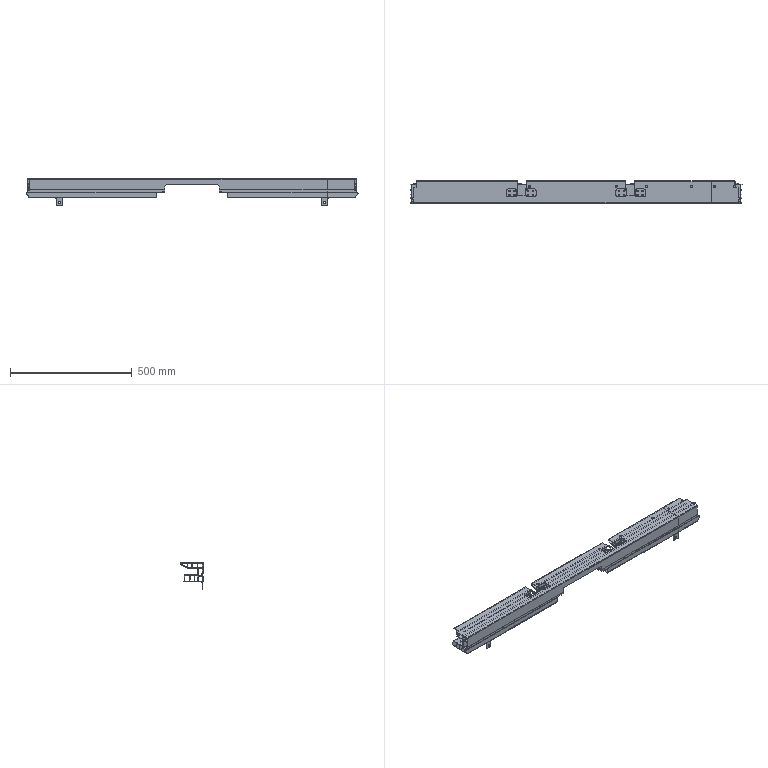NC program | NX | posted with a generic post | part box 1365 x 90.95 x 108.501 mm
Lines 17611 to 18323 of 23380:
(FIXED_CONTOUR , TOOL : R3)
N35190 T09 M6
N35192 G54
N35194 G17 G0 G90 X-536.016 Y-22.112 B0. C0. S9500 M3
N35196 G43 Z30. H9
N35198 Z-6.865
N35200 G94 G1 Z-11.665 F1000.
N35202 X-535.981 Y-22.077 Z-11.732 F2500.
N35204 X-535.904 Y-22. Z-11.861
N35206 X-535.813 Z-12.005
N35208 X-535.883 Y-22.071 Z-11.892
N35210 X-535.962 Y-22.15 Z-11.76
N35212 X-536.034 Y-22.222 Z-11.622
N35214 X-536.044 Y-22.287 Z-11.598
N35216 X-536.049 Y-22.329 Z-11.588
N35218 X-535.992 Y-22.271 Z-11.695
N35220 X-535.943 Y-22.223 Z-11.788
N35222 X-535.816 Y-22.096 Z-12.
N35224 X-535.721 Y-22. Z-12.146
N35226 X-535.696 Z-12.184
N35228 X-535.622 Z-12.282
N35230 X-535.696 Y-22.074 Z-12.182
N35232 X-535.756 Y-22.135 Z-12.087
N35234 X-535.816 Y-22.194 Z-12.
N35236 X-535.931 Y-22.31 Z-11.806
N35238 X-536.061 Y-22.44 Z-11.566
N35240 X-536.062 Y-22.536 Z-11.565
N35242 X-535.932 Y-22.406 Z-11.804
N35244 X-535.816 Y-22.29 Z-12.
N35246 X-535.727 Y-22.201 Z-12.131
N35248 X-535.696 Y-22.17 Z-12.179
N35250 X-535.576 Y-22.05 Z-12.341
N35252 X-535.526 Y-22. Z-12.398
N35254 X-535.427 Z-12.51
N35256 X-535.576 Y-22.149 Z-12.339
N35258 X-535.696 Y-22.269 Z-12.176
N35260 X-535.816 Y-22.389 Z-12.
N35262 X-535.934 Y-22.507 Z-11.802
N35264 X-536.062 Y-22.635 Z-11.564
N35266 Y-22.738
N35268 X-535.935 Y-22.611 Z-11.799
N35270 X-535.816 Y-22.493 Z-12.
N35272 X-535.696 Y-22.373 Z-12.176
N35274 X-535.576 Y-22.252 Z-12.336
N35276 X-535.33 Y-22.006 Z-12.618
N35278 X-535.323 Y-22. Z-12.625
N35280 X-535.213 Z-12.734
N35282 X-535.336 Y-22.122 Z-12.613
N35284 X-535.576 Y-22.362 Z-12.336
N35286 X-535.696 Y-22.483 Z-12.176
N35288 X-535.816 Y-22.603 Z-12.
N35290 X-535.936 Y-22.723 Z-11.797
N35292 X-536.062 Y-22.848 Z-11.564
N35294 Y-22.959 Z-11.563
N35296 X-535.936 Y-22.833 Z-11.796
N35298 X-535.816 Y-22.713 Z-12.
N35300 X-535.696 Y-22.593 Z-12.176
N35302 X-535.576 Y-22.473 Z-12.336
N35304 X-535.336 Y-22.232 Z-12.613
N35306 X-535.226 Y-22.123 Z-12.718
N35308 X-535.103 Y-22. Z-12.843
N35310 X-535.095 Z-12.851
N35312 X-534.993 Z-12.93
N35314 X-535.095 Y-22.102 Z-12.849
N35316 X-535.175 Y-22.182 Z-12.769
N35318 X-535.336 Y-22.343 Z-12.613
N35320 X-535.576 Y-22.583 Z-12.336
N35322 X-535.696 Y-22.703 Z-12.176
N35324 X-535.816 Y-22.823 Z-12.
N35326 X-535.936 Y-22.943 Z-11.796
N35328 X-536.062 Y-23.069 Z-11.563
N35330 Y-23.179 Z-11.564
N35332 X-535.936 Y-23.053 Z-11.796
N35334 X-535.816 Y-22.933 Z-12.
N35336 X-535.696 Y-22.813 Z-12.176
N35338 X-535.576 Y-22.693 Z-12.336
N35340 X-535.336 Y-22.453 Z-12.613
N35342 X-535.095 Y-22.212 Z-12.847
N35344 X-534.883 Y-22. Z-13.016
N35346 X-534.773 Z-13.096
N35348 X-534.855 Y-22.082 Z-13.037
N35350 X-535.095 Y-22.322 Z-12.845
N35352 X-535.336 Y-22.563 Z-12.613
N35354 X-535.576 Y-22.803 Z-12.336
N35356 X-535.696 Y-22.923 Z-12.176
N35358 X-535.816 Y-23.043 Z-12.
N35360 X-535.936 Y-23.163 Z-11.796
N35362 X-536.061 Y-23.289 Z-11.564
N35364 Y-23.398 Z-11.565
N35366 X-535.936 Y-23.273 Z-11.797
N35368 X-535.816 Y-23.153 Z-12.
N35370 X-535.696 Y-23.033 Z-12.176
N35372 X-535.576 Y-22.913 Z-12.336
N35374 X-535.336 Y-22.672 Z-12.613
N35376 X-535.095 Y-22.432 Z-12.845
N35378 X-534.855 Y-22.192 Z-13.037
N35380 X-534.765 Y-22.102 Z-13.1
N35382 X-534.663 Y-21.999 Z-13.175
N35384 X-534.615 Z-13.209
N35386 X-534.553 Z-13.246
N35388 X-534.615 Y-22.061 Z-13.208
N35390 X-534.714 Y-22.16 Z-13.135
N35392 X-534.855 Y-22.301 Z-13.037
N35394 X-535.095 Y-22.541 Z-12.845
N35396 X-535.336 Y-22.782 Z-12.613
N35398 X-535.576 Y-23.022 Z-12.336
N35400 X-535.696 Y-23.142 Z-12.176
N35402 X-535.816 Y-23.262 Z-12.
N35404 X-535.935 Y-23.381 Z-11.799
N35406 X-536.061 Y-23.507 Z-11.566
N35408 Y-23.572
N35410 X-536.058 Y-23.614 Z-11.573
N35412 X-535.934 Y-23.489 Z-11.801
N35414 X-535.816 Y-23.372 Z-12.
N35416 X-535.696 Y-23.252 Z-12.176
N35418 X-535.576 Y-23.132 Z-12.336
N35420 X-535.336 Y-22.891 Z-12.613
N35422 X-535.095 Y-22.651 Z-12.845
N35424 X-534.855 Y-22.411 Z-13.037
N35426 X-534.662 Y-22.218 Z-13.171
N35428 X-534.615 Y-22.17 Z-13.206
N35430 X-534.441 Y-21.997 Z-13.311
N35432 X-534.33 Y-21.996 Z-13.375
N35434 X-534.374 Y-22.04 Z-13.351
N35436 X-534.615 Y-22.28 Z-13.204
N35438 X-534.855 Y-22.521 Z-13.037
N35440 X-535.095 Y-22.761 Z-12.845
N35442 X-535.336 Y-23.001 Z-12.613
N35444 X-535.576 Y-23.241 Z-12.336
N35446 X-535.696 Y-23.362 Z-12.176
N35448 X-535.816 Y-23.482 Z-12.
N35450 X-535.933 Y-23.598 Z-11.803
N35452 X-536.046 Y-23.712 Z-11.594
N35454 X-536.031 Y-23.804 Z-11.63
N35456 X-535.931 Y-23.705 Z-11.805
N35458 X-535.816 Y-23.589 Z-12.
N35460 X-535.696 Y-23.469 Z-12.176
N35462 X-535.576 Y-23.349 Z-12.336
N35464 X-535.336 Y-23.109 Z-12.613
N35466 X-535.095 Y-22.868 Z-12.845
N35468 X-534.855 Y-22.628 Z-13.037
N35470 X-534.615 Y-22.388 Z-13.204
N35472 X-534.374 Y-22.147 Z-13.351
N35474 X-534.304 Y-22.077 Z-13.386
N35476 X-534.221 Y-21.994 Z-13.432
N35478 X-534.134 Y-21.993 Z-13.475
N35480 X-534.11 Y-21.991 Z-13.486
N35482 X-534.219 Y-22.1 Z-13.431
N35484 X-534.254 Y-22.134 Z-13.411
N35486 X-534.374 Y-22.255 Z-13.351
N35488 X-534.615 Y-22.495 Z-13.204
N35490 X-534.855 Y-22.735 Z-13.037
N35492 X-535.095 Y-22.976 Z-12.845
N35494 X-535.336 Y-23.216 Z-12.613
N35496 X-535.576 Y-23.456 Z-12.336
N35498 X-535.696 Y-23.576 Z-12.176
N35500 X-535.816 Y-23.697 Z-12.
N35502 X-535.914 Y-23.795 Z-11.836
N35504 X-535.962 Y-23.842 Z-11.76
N35506 X-536.007 Y-23.887 Z-11.682
N35508 X-536.003 Y-23.899 Z-11.689
N35510 X-535.97 Y-23.96 Z-11.752
N35512 X-535.893 Y-23.883 Z-11.874
N35514 X-535.873 Y-23.863 Z-11.903
N35516 X-535.816 Y-23.806 Z-12.
N35518 X-535.696 Y-23.686 Z-12.176
N35520 X-535.576 Y-23.565 Z-12.336
N35522 X-535.336 Y-23.325 Z-12.613
N35524 X-535.095 Y-23.085 Z-12.845
N35526 X-534.855 Y-22.845 Z-13.037
N35528 X-534.615 Y-22.604 Z-13.204
N35530 X-534.374 Y-22.364 Z-13.351
N35532 X-534.203 Y-22.193 Z-13.436
N35534 X-534.134 Y-22.124 Z-13.473
N35536 X-533.993 Y-21.982 Z-13.54
N35538 X-533.873 Y-21.974 Z-13.589
N35540 X-533.894 Y-21.995 Z-13.581
N35542 X-534.146 Y-22.247 Z-13.465
N35544 X-534.374 Y-22.475 Z-13.351
N35546 X-534.615 Y-22.716 Z-13.204
N35548 X-534.855 Y-22.956 Z-13.037
N35550 X-535.095 Y-23.196 Z-12.845
N35552 X-535.336 Y-23.436 Z-12.613
N35554 X-535.576 Y-23.677 Z-12.336
N35556 X-535.696 Y-23.797 Z-12.178
N35558 X-535.816 Y-23.917 Z-12.
N35560 X-535.841 Y-23.941 Z-11.959
N35562 X-535.899 Y-24. Z-11.869
N35564 X-535.786 Z-12.045
N35566 X-535.696 Y-23.91 Z-12.181
N35568 X-535.576 Y-23.79 Z-12.337
N35570 X-535.336 Y-23.549 Z-12.613
N35572 X-535.095 Y-23.309 Z-12.845
N35574 X-534.855 Y-23.069 Z-13.037
N35576 X-534.615 Y-22.828 Z-13.204
N35578 X-534.374 Y-22.588 Z-13.351
N35580 X-534.109 Y-22.322 Z-13.482
N35582 X-533.894 Y-22.108 Z-13.58
N35584 X-533.751 Y-21.965 Z-13.633
N35586 X-533.653 Y-21.957 Z-13.669
N35588 X-533.617 Y-21.946 Z-13.678
N35590 X-533.653 Y-21.982 Z-13.668
N35592 X-533.894 Y-22.223 Z-13.58
N35594 X-534.134 Y-22.463 Z-13.47
N35596 X-534.374 Y-22.703 Z-13.351
N35598 X-534.615 Y-22.944 Z-13.204
N35600 X-534.855 Y-23.184 Z-13.037
N35602 X-535.095 Y-23.424 Z-12.845
N35604 X-535.336 Y-23.665 Z-12.613
N35606 X-535.492 Y-23.821 Z-12.433
N35608 X-535.576 Y-23.905 Z-12.34
N35610 X-535.671 Y-24. Z-12.217
N35612 X-535.576 Z-12.342
N35614 X-535.563 Z-12.356
N35616 X-535.441 Y-23.878 Z-12.491
N35618 X-535.336 Y-23.772 Z-12.613
N35620 X-535.095 Y-23.532 Z-12.845
N35622 X-534.855 Y-23.292 Z-13.037
N35624 X-534.615 Y-23.051 Z-13.204
N35626 X-534.374 Y-22.811 Z-13.351
N35628 X-534.134 Y-22.571 Z-13.47
N35630 X-533.894 Y-22.33 Z-13.579
N35632 X-533.653 Y-22.09 Z-13.667
N35634 X-533.46 Y-21.897 Z-13.72
N35636 X-533.413 Y-21.882 Z-13.732
N35638 X-533.304 Y-21.849 Z-13.755
N35640 X-533.413 Y-21.958 Z-13.732
N35642 X-533.653 Y-22.198 Z-13.666
N35644 X-533.894 Y-22.439 Z-13.579
N35646 X-534.134 Y-22.679 Z-13.47
N35648 X-534.374 Y-22.919 Z-13.351
N35650 X-534.615 Y-23.16 Z-13.204
N35652 X-534.855 Y-23.4 Z-13.037
N35654 X-535.095 Y-23.64 Z-12.845
N35656 X-535.336 Y-23.881 Z-12.613
N35658 X-535.455 Y-24. Z-12.478
N35660 X-535.348 Z-12.599
N35662 X-535.336 Y-23.988 Z-12.613
N35664 X-535.095 Y-23.747 Z-12.846
N35666 X-534.855 Y-23.507 Z-13.037
N35668 X-534.615 Y-23.267 Z-13.204
N35670 X-534.374 Y-23.026 Z-13.351
N35672 X-534.134 Y-22.786 Z-13.47
N35674 X-533.894 Y-22.546 Z-13.578
N35676 X-533.642 Y-22.294 Z-13.668
N35678 X-533.413 Y-22.065 Z-13.732
N35680 X-533.145 Y-21.797 Z-13.787
N35682 X-533.087 Y-21.774 Z-13.799
N35684 X-532.983 Y-21.733 Z-13.813
N35686 X-533.106 Y-21.856 Z-13.795
N35688 X-533.413 Y-22.163 Z-13.731
N35690 X-533.653 Y-22.403 Z-13.665
N35692 X-533.894 Y-22.644 Z-13.578
N35694 X-534.134 Y-22.884 Z-13.47
N35696 X-534.374 Y-23.124 Z-13.351
N35698 X-534.615 Y-23.365 Z-13.204
N35700 X-534.855 Y-23.605 Z-13.037
N35702 X-535.039 Y-23.789 Z-12.891
N35704 X-535.095 Y-23.845 Z-12.848
N35706 X-535.25 Y-24. Z-12.698
N35708 X-535.151 Z-12.795
N35710 X-535.095 Y-23.944 Z-12.85
N35712 X-534.993 Y-23.841 Z-12.927
N35714 X-534.855 Y-23.703 Z-13.037
N35716 X-534.615 Y-23.463 Z-13.204
N35718 X-534.374 Y-23.223 Z-13.351
N35720 X-534.134 Y-22.983 Z-13.47
N35722 X-533.894 Y-22.742 Z-13.578
N35724 X-533.653 Y-22.502 Z-13.665
N35726 X-533.413 Y-22.262 Z-13.731
N35728 X-533.056 Y-21.904 Z-13.803
N35730 X-532.932 Y-21.781 Z-13.82
N35732 X-532.82 Y-21.668 Z-13.833
N35734 X-532.747 Y-21.637 Z-13.844
N35736 X-532.655 Y-21.596 Z-13.849
N35738 X-532.733 Y-21.675 Z-13.844
N35740 X-532.764 Y-21.705 Z-13.837
N35742 X-532.809 Y-21.751 Z-13.831
N35744 X-532.932 Y-21.874 Z-13.82
N35746 X-533.032 Y-21.974 Z-13.806
N35748 X-533.143 Y-22.084 Z-13.786
N35750 X-533.413 Y-22.355 Z-13.731
N35752 X-533.653 Y-22.595 Z-13.664
N35754 X-533.894 Y-22.835 Z-13.577
N35756 X-534.134 Y-23.076 Z-13.47
N35758 X-534.374 Y-23.316 Z-13.351
N35760 X-534.615 Y-23.556 Z-13.204
N35762 X-534.855 Y-23.797 Z-13.037
N35764 X-534.95 Y-23.891 Z-12.962
N35766 X-535.058 Y-24. Z-12.88
N35768 X-534.965 Z-12.952
N35770 X-534.855 Y-23.89 Z-13.037
N35772 X-534.615 Y-23.65 Z-13.204
N35774 X-534.374 Y-23.41 Z-13.351
N35776 X-534.134 Y-23.169 Z-13.47
N35778 X-533.894 Y-22.929 Z-13.577
N35780 X-533.653 Y-22.689 Z-13.664
N35782 X-533.413 Y-22.448 Z-13.73
N35784 X-533.161 Y-22.196 Z-13.781
N35786 X-533.009 Y-22.044 Z-13.809
N35788 X-532.932 Y-21.968 Z-13.82
N35790 X-532.719 Y-21.755 Z-13.84
N35792 X-532.708 Y-21.743 Z-13.842
N35794 X-532.591 Y-21.626 Z-13.85
N35796 X-532.492 Y-21.527
N35798 X-532.452 Y-21.511
N35800 X-532.379 Y-21.542 Z-13.849
N35802 X-532.532 Y-21.695 Z-13.85
N35804 X-532.692 Y-21.855 Z-13.842
N35806 X-532.932 Y-22.096 Z-13.82
N35808 X-532.977 Y-22.14 Z-13.814
N35810 X-533.173 Y-22.336 Z-13.778
N35812 X-533.413 Y-22.576 Z-13.729
N35814 X-533.653 Y-22.816 Z-13.664
N35816 X-533.894 Y-23.057 Z-13.576
N35818 X-534.134 Y-23.297 Z-13.47
N35820 X-534.374 Y-23.537 Z-13.351
N35822 X-534.615 Y-23.778 Z-13.205
N35824 X-534.837 Y-24. Z-13.05
N35826 X-534.709 Z-13.142
N35828 X-534.615 Y-23.906 Z-13.207
N35830 X-534.53 Y-23.821 Z-13.256
N35832 X-534.374 Y-23.666 Z-13.351
N35834 X-534.134 Y-23.425 Z-13.47
N35836 X-533.894 Y-23.185 Z-13.575
N35838 X-533.653 Y-22.945 Z-13.664
N35840 X-533.413 Y-22.704 Z-13.728
N35842 X-533.173 Y-22.464 Z-13.778
N35844 X-532.932 Y-22.224 Z-13.82
N35846 X-532.692 Y-21.983 Z-13.842
N35848 X-532.452 Y-21.743 Z-13.85
N35850 X-532.289 Y-21.58 Z-13.849
N35852 X-532.197 Y-21.619 Z-13.847
N35854 X-532.452 Y-21.874 Z-13.85
N35856 X-532.692 Y-22.114 Z-13.842
N35858 X-532.932 Y-22.354 Z-13.82
N35860 X-533.226 Y-22.648 Z-13.766
N35862 X-533.413 Y-22.835 Z-13.727
N35864 X-533.653 Y-23.075 Z-13.663
N35866 X-533.894 Y-23.315 Z-13.575
N35868 X-534.134 Y-23.556 Z-13.47
N35870 X-534.374 Y-23.796 Z-13.351
N35872 X-534.469 Y-23.891 Z-13.293
N35874 X-534.578 Y-24. Z-13.23
N35876 X-534.447 Z-13.308
N35878 X-534.374 Y-23.927 Z-13.351
N35880 X-534.134 Y-23.687 Z-13.47
N35882 X-533.894 Y-23.447 Z-13.574
N35884 X-533.653 Y-23.206 Z-13.663
N35886 X-533.413 Y-22.966 Z-13.727
N35888 X-533.173 Y-22.726 Z-13.777
N35890 X-532.932 Y-22.485 Z-13.819
N35892 X-532.692 Y-22.245 Z-13.842
N35894 X-532.452 Y-22.005 Z-13.85
N35896 X-532.199 Y-21.752 Z-13.842
N35898 X-532.106 Y-21.659 Z-13.836
N35900 X-532.011 Y-21.697 Z-13.825
N35902 X-532.212 Y-21.898 Z-13.842
N35904 X-532.452 Y-22.138 Z-13.85
N35906 X-532.692 Y-22.378 Z-13.842
N35908 X-532.932 Y-22.619 Z-13.819
N35910 X-533.173 Y-22.859 Z-13.777
N35912 X-533.413 Y-23.099 Z-13.726
N35914 X-533.653 Y-23.339 Z-13.663
N35916 X-533.894 Y-23.58 Z-13.573
N35918 X-534.089 Y-23.775 Z-13.489
N35920 X-534.134 Y-23.82 Z-13.472
N35922 X-534.314 Y-24. Z-13.384
N35924 X-534.18 Z-13.452
N35926 X-534.134 Y-23.954 Z-13.474
N35928 X-534.027 Y-23.847 Z-13.515
N35930 X-533.894 Y-23.713 Z-13.573
N35932 X-533.653 Y-23.473 Z-13.662
N35934 X-533.413 Y-23.233 Z-13.726
N35936 X-533.173 Y-22.992 Z-13.777
N35938 X-533.094 Y-22.914 Z-13.789
N35940 X-532.932 Y-22.752 Z-13.819
N35942 X-532.692 Y-22.512 Z-13.842
N35944 X-532.452 Y-22.271 Z-13.85
N35946 X-532.212 Y-22.031 Z-13.842
N35948 X-531.971 Y-21.791 Z-13.82
N35950 X-531.915 Y-21.735 Z-13.812
N35952 X-531.818 Y-21.773 Z-13.799
N35954 X-531.971 Y-21.927 Z-13.819
N35956 X-532.212 Y-22.167 Z-13.842
N35958 X-532.452 Y-22.407 Z-13.85
N35960 X-532.692 Y-22.648 Z-13.842
N35962 X-532.932 Y-22.888 Z-13.817
N35964 X-533.049 Y-23.005 Z-13.796
N35966 X-533.173 Y-23.128 Z-13.777
N35968 X-533.413 Y-23.369 Z-13.725
N35970 X-533.653 Y-23.609 Z-13.662
N35972 X-533.894 Y-23.849 Z-13.572
N35974 X-533.964 Y-23.919 Z-13.542
N35976 X-534.044 Y-24. Z-13.511
N35978 X-533.908 Z-13.566
N35980 X-533.653 Y-23.745 Z-13.661
N35982 X-533.413 Y-23.505 Z-13.725
N35984 X-533.173 Y-23.264 Z-13.777
N35986 X-533.004 Y-23.095 Z-13.803
N35988 X-532.932 Y-23.024 Z-13.816
N35990 X-532.843 Y-22.935 Z-13.827
N35992 X-532.692 Y-22.784 Z-13.841
N35994 X-532.452 Y-22.543 Z-13.85
N35996 X-532.212 Y-22.303 Z-13.842
N35998 X-531.971 Y-22.063 Z-13.819
N36000 X-531.794 Y-21.885 Z-13.794
N36002 X-531.72 Y-21.812 Z-13.779
N36004 X-531.615 Y-21.844 Z-13.758
N36006 X-531.775 Y-22.003 Z-13.789
N36008 X-531.971 Y-22.2 Z-13.818
N36010 X-532.212 Y-22.44 Z-13.842
N36012 X-532.452 Y-22.68 Z-13.85
N36014 X-532.692 Y-22.921 Z-13.841
N36016 X-532.798 Y-23.026 Z-13.831
N36018 X-532.932 Y-23.161 Z-13.815
N36020 X-533.173 Y-23.401 Z-13.777
N36022 X-533.413 Y-23.641 Z-13.725
N36024 X-533.653 Y-23.882 Z-13.662
N36026 X-533.772 Y-24. Z-13.618
N36028 X-533.653 Z-13.662
N36030 X-533.634 Z-13.667
N36032 X-533.413 Y-23.779 Z-13.724
N36034 X-533.173 Y-23.539 Z-13.777
N36036 X-532.932 Y-23.298 Z-13.814
N36038 X-532.692 Y-23.058 Z-13.841
N36040 X-532.452 Y-22.818 Z-13.849
N36042 X-532.212 Y-22.578 Z-13.842
N36044 X-531.971 Y-22.337 Z-13.818
N36046 X-531.755 Y-22.121 Z-13.784
N36048 X-531.51 Y-21.876 Z-13.737
N36050 X-531.404 Y-21.909 Z-13.71
N36052 X-531.491 Y-21.996 Z-13.732
N36054 X-531.766 Y-22.271 Z-13.784
N36056 X-531.971 Y-22.476 Z-13.818
N36058 X-532.212 Y-22.717 Z-13.842
N36060 X-532.452 Y-22.957 Z-13.849
N36062 X-532.706 Y-23.211 Z-13.839
N36064 X-532.932 Y-23.438 Z-13.814
N36066 X-533.188 Y-23.693 Z-13.773
N36068 X-533.413 Y-23.918 Z-13.724
N36070 X-533.495 Y-24. Z-13.704
N36072 X-533.356 Z-13.737
N36074 X-533.173 Y-23.817 Z-13.778
N36076 X-532.932 Y-23.576 Z-13.814
N36078 X-532.692 Y-23.336 Z-13.841
N36080 X-532.452 Y-23.096 Z-13.849
N36082 X-532.212 Y-22.855 Z-13.841
N36084 X-531.971 Y-22.615 Z-13.818
N36086 X-531.731 Y-22.375 Z-13.778
N36088 X-531.491 Y-22.135 Z-13.732
N36090 X-531.298 Y-21.942 Z-13.682
N36092 X-531.248 Y-21.958 Z-13.668
N36094 X-531.183 Y-21.963 Z-13.644
N36096 X-531.25 Y-22.03 Z-13.668
N36098 X-531.346 Y-22.125 Z-13.692
N36100 X-531.491 Y-22.271 Z-13.731
N36102 X-531.731 Y-22.511 Z-13.778
N36104 X-531.971 Y-22.751 Z-13.818
N36106 X-532.212 Y-22.991 Z-13.841
N36108 X-532.452 Y-23.232 Z-13.849
N36110 X-532.692 Y-23.472 Z-13.841
N36112 X-532.932 Y-23.712 Z-13.814
N36114 X-533.066 Y-23.846 Z-13.793
N36116 X-533.097 Y-23.877 Z-13.791
N36118 X-533.173 Y-23.953 Z-13.78
N36120 X-533.22 Y-24. Z-13.77
N36122 X-533.173 Z-13.781
N36124 X-533.084 Z-13.795
N36126 X-533.003 Y-23.919 Z-13.803
N36128 X-532.933 Y-23.848 Z-13.814
N36130 X-532.692 Y-23.608 Z-13.841
N36132 X-532.452 Y-23.367 Z-13.849
N36134 X-532.33 Y-23.246 Z-13.846
N36136 X-532.212 Y-23.127 Z-13.84
N36138 X-531.971 Y-22.887 Z-13.817
N36140 X-531.731 Y-22.646 Z-13.777
N36142 X-531.491 Y-22.406 Z-13.73
N36144 X-531.25 Y-22.165 Z-13.666
N36146 X-531.056 Y-21.972 Z-13.598
N36148 X-531.01 Y-21.975 Z-13.581
N36150 X-530.93 Y-21.981 Z-13.548
N36152 X-531.01 Y-22.061 Z-13.58
N36154 X-531.25 Y-22.302 Z-13.665
N36156 X-531.491 Y-22.542 Z-13.729
N36158 X-531.757 Y-22.809 Z-13.781
N36160 X-531.971 Y-23.022 Z-13.816
N36162 X-532.212 Y-23.263 Z-13.839
N36164 X-532.332 Y-23.383 Z-13.846
N36166 X-532.452 Y-23.503 Z-13.849
N36168 X-532.692 Y-23.743 Z-13.841
N36170 X-532.949 Y-24. Z-13.812
N36172 X-532.815 Z-13.829
N36174 X-532.692 Y-23.877 Z-13.843
N36176 X-532.621 Y-23.806
N36178 X-532.452 Y-23.637 Z-13.849
N36180 X-532.277 Y-23.462 Z-13.843
N36182 X-532.212 Y-23.397 Z-13.84
N36184 X-531.971 Y-23.156 Z-13.815
N36186 X-531.731 Y-22.916 Z-13.777
N36188 X-531.491 Y-22.676 Z-13.728
N36190 X-531.25 Y-22.436 Z-13.664
N36192 X-531.01 Y-22.195 Z-13.579
N36194 X-530.918 Y-22.103 Z-13.538
N36196 X-530.875 Y-22.06 Z-13.522
N36198 X-530.805 Y-21.99 Z-13.491
N36200 X-530.766 Y-21.993 Z-13.473
N36202 X-530.681 Y-21.994 Z-13.429
N36204 X-530.77 Y-22.083 Z-13.474
N36206 X-530.858 Y-22.171 Z-13.511
N36208 X-531.01 Y-22.323 Z-13.578
N36210 X-531.25 Y-22.564 Z-13.664
N36212 X-531.491 Y-22.804 Z-13.727
N36214 X-531.731 Y-23.044 Z-13.777
N36216 X-531.971 Y-23.285 Z-13.814
N36218 X-532.212 Y-23.525 Z-13.84
N36220 X-532.332 Y-23.645 Z-13.846
N36222 X-532.452 Y-23.765 Z-13.849
N36224 X-532.561 Y-23.874 Z-13.845
N36226 X-532.599 Y-23.912 Z-13.847
N36228 X-532.687 Y-24. Z-13.845
N36230 X-532.557 Z-13.85
N36232 X-532.501 Y-23.944 Z-13.847
N36234 X-532.452 Y-23.895 Z-13.849
N36236 X-532.212 Y-23.655 Z-13.84
N36238 X-531.971 Y-23.414 Z-13.814
N36240 X-531.731 Y-23.174 Z-13.777
N36242 X-531.491 Y-22.934 Z-13.727
N36244 X-531.25 Y-22.693 Z-13.664
N36246 X-531.01 Y-22.453 Z-13.578
N36248 X-530.769 Y-22.212 Z-13.471
N36250 X-530.553 Y-21.996 Z-13.363
N36252 X-530.525 Z-13.349
N36254 X-530.426 Y-21.998 Z-13.29
N36256 X-530.529 Y-22.101 Z-13.351
N36258 X-530.77 Y-22.341 Z-13.471
N36260 X-531.01 Y-22.582 Z-13.577
N36262 X-531.25 Y-22.822 Z-13.664
N36264 X-531.491 Y-23.062 Z-13.726
N36266 X-531.731 Y-23.303 Z-13.777
N36268 X-531.971 Y-23.543 Z-13.814
N36270 X-532.212 Y-23.783 Z-13.841
N36272 X-532.428 Y-24. Z-13.849
N36274 X-532.302 Z-13.846
N36276 X-532.212 Y-23.91 Z-13.843
N36278 X-532.125 Y-23.823 Z-13.831
N36280 X-531.971 Y-23.669 Z-13.814
N36282 X-531.731 Y-23.429 Z-13.777
N36284 X-531.491 Y-23.189 Z-13.726
N36286 X-531.25 Y-22.949 Z-13.663
N36288 X-531.01 Y-22.708 Z-13.577
N36290 X-530.77 Y-22.468 Z-13.471
N36292 X-530.529 Y-22.228 Z-13.351
N36294 X-530.42 Y-22.119 Z-13.284
N36296 X-530.301 Y-21.999 Z-13.216
N36298 X-530.184 Y-22. Z-13.134
N36300 X-530.289 Y-22.105 Z-13.207
N36302 X-530.366 Y-22.182 Z-13.251
N36304 X-530.529 Y-22.345 Z-13.351
N36306 X-530.77 Y-22.586 Z-13.471
N36308 X-531.01 Y-22.826 Z-13.576
N36310 X-531.25 Y-23.066 Z-13.663
N36312 X-531.491 Y-23.307 Z-13.725
N36314 X-531.731 Y-23.547 Z-13.777
N36316 X-531.971 Y-23.787 Z-13.814
N36318 X-532.07 Y-23.886 Z-13.825
N36320 X-532.184 Y-24. Z-13.841
N36322 X-532.062 Z-13.826
N36324 X-531.971 Y-23.909 Z-13.814
N36326 X-531.731 Y-23.669 Z-13.777
N36328 X-531.491 Y-23.429 Z-13.725
N36330 X-531.25 Y-23.188 Z-13.663
N36332 X-531.01 Y-22.948 Z-13.576
N36334 X-530.77 Y-22.708 Z-13.471
N36336 X-530.529 Y-22.468 Z-13.351
N36338 X-530.288 Y-22.226 Z-13.204
N36340 X-530.062 Y-22. Z-13.047
N36342 X-529.941 Z-12.954
N36344 X-530.049 Y-22.108 Z-13.037
N36346 X-530.289 Y-22.348 Z-13.204
N36348 X-530.529 Y-22.589 Z-13.351
N36350 X-530.77 Y-22.829 Z-13.471
N36352 X-531.01 Y-23.069 Z-13.575
N36354 X-531.25 Y-23.309 Z-13.662
N36356 X-531.491 Y-23.55 Z-13.725
N36358 X-531.731 Y-23.79 Z-13.778
N36360 X-531.941 Y-24. Z-13.81
N36362 X-531.822 Z-13.795
N36364 X-531.73 Y-23.908 Z-13.779
N36366 X-531.645 Y-23.823 Z-13.758
N36368 X-531.491 Y-23.669 Z-13.724
N36370 X-531.25 Y-23.429 Z-13.662
N36372 X-531.01 Y-23.188 Z-13.575
N36374 X-530.77 Y-22.948 Z-13.471
N36376 X-530.529 Y-22.708 Z-13.351
N36378 X-530.289 Y-22.467 Z-13.204
N36380 X-530.049 Y-22.227 Z-13.037
N36382 X-529.941 Y-22.12 Z-12.951
N36384 X-529.822 Y-22. Z-12.862
N36386 X-529.803 Z-12.845
N36388 X-529.716 Z-12.759
N36390 X-529.808 Y-22.093 Z-12.849
N36392 X-529.892 Y-22.176 Z-12.912
N36394 X-530.049 Y-22.333 Z-13.037
N36396 X-530.289 Y-22.574 Z-13.204
N36398 X-530.529 Y-22.814 Z-13.351
N36400 X-530.77 Y-23.054 Z-13.471
N36402 X-531.01 Y-23.295 Z-13.574
N36404 X-531.25 Y-23.535 Z-13.662
N36406 X-531.491 Y-23.775 Z-13.724
N36408 X-531.595 Y-23.88 Z-13.747
N36410 X-531.715 Y-24. Z-13.777
N36412 X-531.606 Z-13.751
N36414 X-531.491 Y-23.885 Z-13.724
N36416 X-531.25 Y-23.644 Z-13.662
N36418 X-531.01 Y-23.404 Z-13.574
N36420 X-530.77 Y-23.164 Z-13.471
N36422 X-530.529 Y-22.923 Z-13.351
N36424 X-530.289 Y-22.683 Z-13.204
N36426 X-530.049 Y-22.443 Z-13.037
N36428 X-529.808 Y-22.202 Z-12.847
N36430 X-529.606 Y-22. Z-12.651
N36432 X-529.565 Z-12.609
N36434 X-529.501 Z-12.538
N36436 X-529.568 Y-22.067 Z-12.613
N36438 X-529.808 Y-22.307 Z-12.845
N36440 X-530.049 Y-22.547 Z-13.037
N36442 X-530.289 Y-22.788 Z-13.204
N36444 X-530.529 Y-23.028 Z-13.351
N36446 X-530.77 Y-23.268 Z-13.471
N36448 X-531.01 Y-23.509 Z-13.573
N36450 X-531.25 Y-23.749 Z-13.661
N36452 X-531.501 Y-24. Z-13.726
N36454 X-531.393 Z-13.7
N36456 X-531.25 Y-23.858 Z-13.662
N36458 X-531.01 Y-23.617 Z-13.573
N36460 X-530.77 Y-23.377 Z-13.471
N36462 X-530.529 Y-23.137 Z-13.351
N36464 X-530.289 Y-22.896 Z-13.204
N36466 X-530.049 Y-22.656 Z-13.037
N36468 X-529.808 Y-22.416 Z-12.845
N36470 X-529.568 Y-22.175 Z-12.613
N36472 X-529.485 Y-22.092 Z-12.517
N36474 X-529.393 Y-22. Z-12.415
N36476 X-529.321 Z-12.334
N36478 X-529.286 Z-12.287
N36480 X-529.328 Y-22.042 Z-12.341
N36482 X-529.435 Y-22.149 Z-12.459
N36484 X-529.568 Y-22.283 Z-12.613
N36486 X-529.808 Y-22.523 Z-12.845
N36488 X-530.049 Y-22.763 Z-13.037
N36490 X-530.289 Y-23.004 Z-13.204
N36492 X-530.529 Y-23.244 Z-13.351
N36494 X-530.77 Y-23.484 Z-13.471
N36496 X-531.009 Y-23.723 Z-13.572
N36498 X-531.25 Y-23.965 Z-13.662
N36500 X-531.286 Y-24. Z-13.672
N36502 X-531.248 Z-13.662
N36504 X-531.188 Z-13.639
N36506 X-531.01 Y-23.822 Z-13.572
N36508 X-530.77 Y-23.582 Z-13.471
N36510 X-530.529 Y-23.341 Z-13.351
N36512 X-530.289 Y-23.101 Z-13.204
N36514 X-530.049 Y-22.861 Z-13.037
N36516 X-529.808 Y-22.621 Z-12.845
N36518 X-529.568 Y-22.38 Z-12.613
N36520 X-529.389 Y-22.201 Z-12.406
N36522 X-529.328 Y-22.14 Z-12.339
N36524 X-529.208 Y-22.02 Z-12.183
N36526 X-529.188 Y-22. Z-12.154
N36528 X-529.091 Z-12.005
N36530 X-529.208 Y-22.117 Z-12.181
N36532 X-529.328 Y-22.237 Z-12.337
N36534 X-529.568 Y-22.477 Z-12.613
N36536 X-529.808 Y-22.718 Z-12.845
N36538 X-530.049 Y-22.958 Z-13.037
N36540 X-530.289 Y-23.198 Z-13.204
N36542 X-530.529 Y-23.439 Z-13.351
N36544 X-530.77 Y-23.679 Z-13.471
N36546 X-531.01 Y-23.919 Z-13.572
N36548 X-531.091 Y-24. Z-13.602
N36550 X-530.995 Z-13.566
N36552 X-530.769 Y-23.774 Z-13.471
N36554 X-530.529 Y-23.534 Z-13.351
N36556 X-530.289 Y-23.294 Z-13.204
N36558 X-530.049 Y-23.054 Z-13.037
N36560 X-529.808 Y-22.813 Z-12.845
N36562 X-529.568 Y-22.573 Z-12.613
N36564 X-529.328 Y-22.333 Z-12.336
N36566 X-529.208 Y-22.213 Z-12.178
N36568 X-529.088 Y-22.092 Z-12.
N36570 X-529.06 Y-22.065 Z-11.953
N36572 X-529.029 Y-22.034 Z-11.908
N36574 X-528.995 Y-22. Z-11.854
N36576 X-528.911 Z-11.716
N36578 X-528.908 Y-22.013 Z-11.71
N36580 X-529.01 Y-22.115 Z-11.873
N36582 X-529.03 Y-22.136 Z-11.903
N36584 X-529.088 Y-22.193 Z-12.
N36586 X-529.208 Y-22.313 Z-12.176
N36588 X-529.328 Y-22.434 Z-12.336
N36590 X-529.568 Y-22.674 Z-12.613
N36592 X-529.808 Y-22.914 Z-12.845
N36594 X-530.049 Y-23.155 Z-13.037
N36596 X-530.289 Y-23.395 Z-13.204
N36598 X-530.529 Y-23.635 Z-13.351
N36600 X-530.699 Y-23.805 Z-13.435
N36602 X-530.77 Y-23.875 Z-13.473
N36604 X-530.894 Y-24. Z-13.525
N36606 X-530.787 Z-13.482
N36608 X-530.77 Y-23.983 Z-13.475